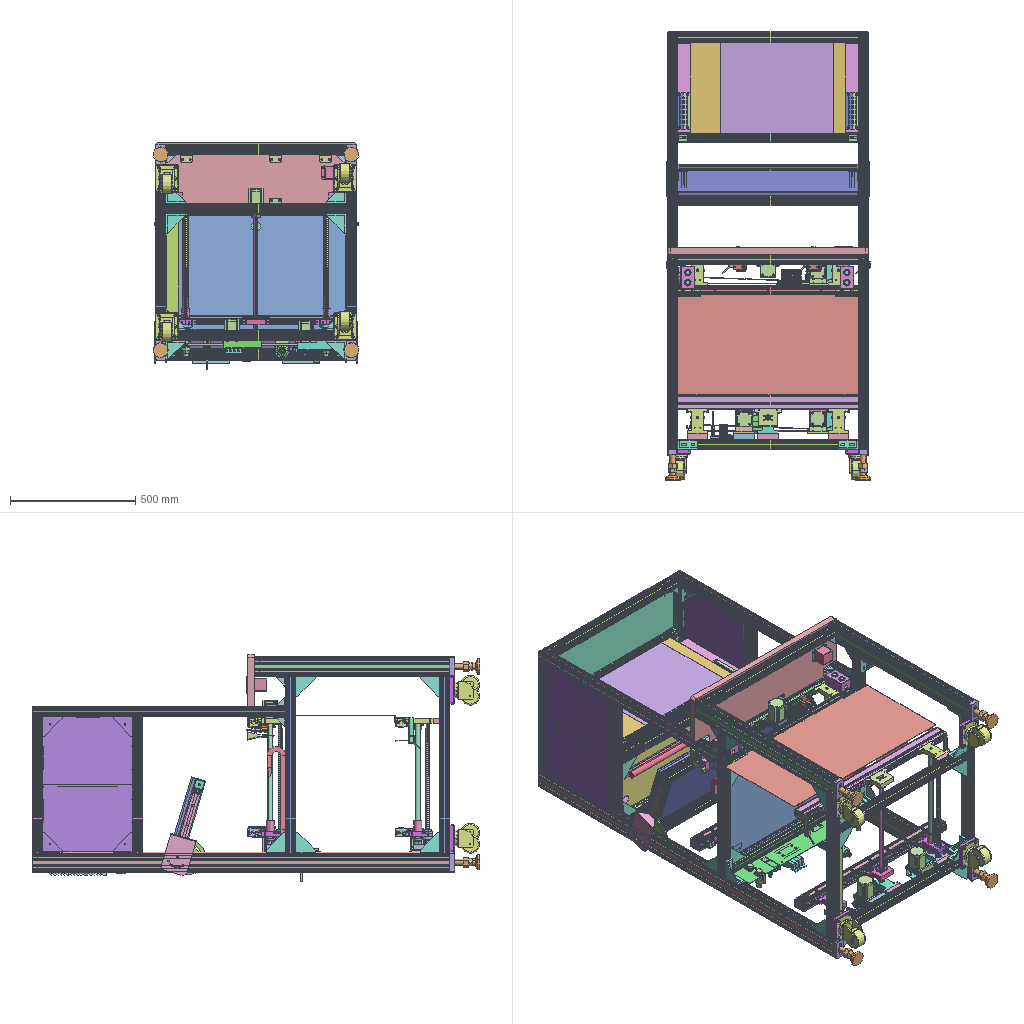Assembly | STEP file | 164 different items | 883 placed | box 820 x 1786 x 902 mm
Parts list (item | name | quantity | parent item | size | volume):
1 | MK-8-4080H-L-02 profile 4080H standard type 1620mm | x2 | in Aluminium profile frame assembly 2 | 1664 x 40 x 80 mm | 1350750 mm3
2 | MK-8-4040C-L-00 profile 4040C standard type 700mm | x4 | in Aluminium profile frame assembly 2 | 700 x 40 x 40 mm | 334774 mm3
3 | MK-8-4040C-L-00 profile 4040C standard type 720mm | x10 | in Aluminium profile frame assembly 2 | 720 x 40 x 40 mm | 344339 mm3
4 | MK-8-4040C-L-00 profile 4040C standard type 540mm | x4 | in Aluminium profile frame assembly 2 | 540 x 40 x 40 mm | 258254 mm3
5 | Die-cast aluminium connector, 40 series, 40mm face, reinforced type | x34 | in Aluminium profile frame assembly 2 | 78 x 78 x 36 mm | 52626 mm3
6 | All-carbon-steel swivel foot KCUF M24-150-60 | x4 | in Aluminium profile frame assembly 2 | 60 x 195 x 60 mm | 136685 mm3
7 | Foot mounting block | x4 | in Aluminium profile frame assembly 2 | 80 x 40 x 20 mm | 52813 mm3
8 | MK-8-4080H-L-02 profile 4080H standard type 735mm | x2 | in Aluminium profile frame assembly 2 | 779 x 40 x 80 mm | 632330 mm3
9 | MK-8-4040C-L-00 profile 4040C standard type 1010mm | x2 | in Aluminium profile frame assembly 2 | 1010 x 40 x 40 mm | 483031 mm3
10 | Die-cast aluminium connector, 40 series, 40mm face, standard type | x18 | in Aluminium profile frame assembly 2 | 38 x 38 x 36 mm | 14409 mm3
11 | 3 inch heavy-duty caster 7223-222B | x4 | in Aluminium profile frame assembly 2 | 112 x 105 x 88 mm | 158459 mm3
12 | Caster mounting plate | x4 | in Aluminium profile frame assembly 2 | 110 x 90 x 14 mm | 130540 mm3
13 | Left door panel | x1 | in Left sheet-metal door assembly | 362.8 x 357 x 19 mm | 160795 mm3
14 | Hinge CL237Z3H001-01 | x4 | in Hinge CL237Z3H001 | 17.5 x 48 x 18 mm | 5234 mm3
15 | Hinge CL237Z3H001-02 | x4 | in Hinge CL237Z3H001 | 19 x 25 x 8.5 mm | 1495 mm3
16 | Power knob mounting sheet metal | x1 | in Left sheet-metal door assembly | 74 x 122 x 41 mm | 24069 mm3
17 | Right door panel | x1 | in Right door welded assembly | 356 x 357 x 17 mm | 169245 mm3
18 | Door hinge mounting plate | x4 | in Frame assembly | 50 x 53 x 16 mm | 6575 mm3
19 | Tabletop mounting plate A | x3 | in Frame assembly | 30 x 36 x 45 mm | 7668 mm3
20 | Cabinet sheet-metal cover plate A | x2 | in Frame assembly | 358 x 30 x 538 mm | 310725 mm3
21 | Power strip mounting plate | x1 | in Frame assembly | 100 x 719 x 60 mm | 188882 mm3
22 | Tabletop plate | x1 | in Frame assembly | 800 x 250 x 27 mm | 5242609 mm3
23 | Lower support plate 1 | x1 | in Frame assembly | 720 x 462 x 30 mm | 565820 mm3
24 | Lower support plate 2 | x1 | in Frame assembly | 52 x 462 x 30 mm | 48079 mm3
25 | Cabinet sheet-metal cover plate B | x1 | in Frame assembly | 794.836 x 358 x 15 mm | 451787 mm3
26 | Top cover plate | x1 | in Frame assembly | 790 x 1.5 x 650 mm | 765787 mm3
27 | Cylinder lock MS813-Shengjiu | x1 | in Frame assembly | 58.793 x 35 x 31.6 mm | 16415 mm3
28 | Class B ventilation filter set ZL-803 (7032 glue) | x2 | in Frame assembly | 150 x 150 x 28 mm | 421271 mm3
29 | Cabinet lower base plate | x1 | in Frame assembly | 718 x 30 x 268 mm | 336091 mm3
30 | Sheet-metal door stop plate | x1 | in Frame assembly | 15.5 x 36.5 x 150 mm | 10828 mm3
31 | Tabletop mounting plate B | x1 | in Frame assembly | 55 x 31 x 45 mm | 10250 mm3
32 | Line stopper plate | x1 | in Frame assembly | 800 x 431 x 30 mm | 516055 mm3
33 | Cabinet brush KEL-BES-S24 | x2 | in Frame assembly | 148 x 10 x 58 mm | 60298 mm3
34 | Electrical mounting plate | x1 | in Control cabinet | 790 x 360 x 20 mm | 612037 mm3
35 | Straight-through terminal block PT2,5-QUATTRO-3209578 | x28 | in Control cabinet | 5.15 x 72.2 x 35.25 mm | 9561 mm3
36 | End clamp-E UK-1201442 | x1 | in Control cabinet | 50.5 x 35.3 x 9.5 mm | 9735 mm3
37 | Miniature circuit breaker IC65N-2P-C16A | x1 | in Control cabinet | 35.4 x 93.9 x 74.3 mm | 159125 mm3
38 | Residual current device Vigi-iC65-ELE-2P-40A-30mA-A | x1 | in Control cabinet | 76.2 x 105.618 x 73.908 mm | 172404 mm3
39 | Power line filter 3ACA5-W33 | x1 | in Control cabinet | 53.2 x 24 x 50 mm | 35444 mm3
40 | Ultra-miniature medium-power relay HF41F_24-ZST and socket 41F-1Z-C2-1 | x1 | in Control cabinet | 88 x 75.5 x 6.1 mm | 25363 mm3
41 | PLC module FX5U-32MT_ES | x1 | in Control cabinet | 150 x 96.4 x 84.9 mm | 980252 mm3
42 | Stepper motor driver DM542-KK V3.0 | x6 | in Control cabinet | 119 x 77.6 x 25.5 mm | 99944 mm3
43 | Cable trough 4 | x2 | in Control cabinet | 50.625 x 25 x 690 mm | 86789 mm3
44 | Cable trough 5 | x2 | in Control cabinet | 50.625 x 25 x 346 mm | 43498 mm3
45 | Power switch LW42B2-1824_L | x1 | in Control cabinet | 65.5 x 92 x 65.5 mm | 250369 mm3
46 | Indicator light AD17-22-AC220VW white | x1 | in Control cabinet | 24 x 37.7 x 24 mm | 7790 mm3
47 | Power supply mounting plate | x2 | in Control cabinet | 65 x 200 x 20 mm | 18055 mm3
48 | Switching power supply LRS-350-24 | x1 | in Control cabinet | 215 x 30 x 115 mm | 695683 mm3
49 | Switching power supply LRS-350-48 | x1 | in Control cabinet | 215 x 30 x 115 mm | 698035 mm3
50 | Primary busbar bracket JTN1 | x2 | in Control cabinet | 20 x 50 x 65 mm | 42874 mm3
51 | Ground copper plate | x1 | in Control cabinet | 30 x 200 x 5 mm | 28923 mm3
52 | Axial fan 1238A2MBL | x1 | in Control cabinet | 120 x 120 x 38 mm | 111801 mm3
53 | Schneider miniature circuit breaker iDPNN-1P+N-C10A | x1 | in Control cabinet | 17.5 x 90.6 x 73.848 mm | 76092 mm3
54 | Schneider AC contactor (coil 24V) LC1D09BDC | x1 | in Control cabinet | - | -
55 | 5-port DIN-rail switch EDS-205 | x1 | in Control cabinet | 98.5 x 110.5 x 24.9 mm | 215104 mm3
56 | Fuse terminal block PT4-HESILED24(5x20)-3211903 | x2 | in Control cabinet | 6.15 x 55.9 x 63.38 mm | 12999 mm3
57 | BZJ-LSX-RGX PLC扩展IO FX5-16ET_ES8(输入,8输出,晶体管漏型) | x1 | in Control cabinet | 40 x 90 x 83 mm | 291482 mm3
58 | Circuit board assembly | x2 | in Control cabinet | 54 x 38 x 11.5 mm | 8666 mm3
59 | T8 integrated LED tube_white 0.6m | x1 | - | 34 x 35.5 x 620 mm | 542828 mm3
60 | Small support plate_sand-blasted, oxidised | x4 | in Forward-flow width-adjust assembly_chain | 20 x 80 x 80 mm | 64176 mm3
61 | Large support plate_sand-blasted, oxidised | x4 | in Forward-flow width-adjust assembly_chain | 20 x 97 x 80 mm | 92738 mm3
62 | Movable support plate_sand-blasted, oxidised | x4 | in Forward-flow width-adjust assembly_chain | 20 x 95 x 90 mm | 73168 mm3
63 | Guide rod | x4 | in Forward-flow width-adjust assembly_chain | 20 x 20 x 505 mm | 158440 mm3
64 | 6001Z bearing stop plate | x4 | in Forward-flow width-adjust assembly_chain | 40 x 28 x 2 mm | 1349 mm3
65 | Bearing stop plate | x5 | in Forward-flow width-adjust assembly_chain, Line single-drive assembly | 40 x 30 x 2 mm | 1364 mm3
66 | Bearing 6000Z_P5_BONA_eco | x5 | in Forward-flow width-adjust assembly_chain, Line single-drive assembly | 26 x 26 x 8 mm | 2544 mm3
67 | Guided double-liner flanged linear bearing LML21-d20 | x4 | in Forward-flow width-adjust assembly_chain | 80 x 54 x 38 mm | 45928 mm3
68 | Nut SFU01604-4 | x4 | in 69 | 40 x 40 x 48 mm | 25660 mm3
69 | Ball screw assembly SFUR1604-545 | x4 | in 69 | 16 x 16 x 545 mm | 99221 mm3
70 | Bearing 6001ZZ | x5 | in Forward-flow width-adjust assembly_chain, Line single-drive assembly | 28 x 28 x 8 mm | 3776 mm3
71 | Locking bearing nut BKN21-M12 (M12×1.0)_yhda | x4 | in Forward-flow width-adjust assembly_chain | 22 x 22 x 8 mm | 1773 mm3
72 | Timing pulley 24-3M-φ10-23 | x4 | in Forward-flow width-adjust assembly_chain | 25 x 23 x 25 mm | 7405 mm3
73 | Motor adapter plate 2 | x2 | in Chain conveyor | 110 x 21 x 64 mm | 49771 mm3
74 | - | x8 | in BZJ-LSX-RGX 链条惰轮Component-30 | 31 x 9 x 31 mm | 3611 mm3
75 | Deep groove ball bearing 606-2Z | x16 | in BZJ-LSX-RGX 链条惰轮Component-30, BZJ-LSX-RGX 链条惰轮Component-25 | 6 x 17 x 17 mm | 776.566 mm3
76 | Internal retaining ring type A 17 | x16 | in BZJ-LSX-RGX 链条惰轮Component-30, BZJ-LSX-RGX 链条惰轮Component-25 | 18.3 x 17.603 x 1 mm | 85.781 mm3
77 | Sprocket spacer | x8 | in Chain conveyor, Line single-drive assembly | 15 x 15 x 6.2 mm | 541.108 mm3
78 | Line rear chain guide rail L800 | x2 | in Chain conveyor, Chain conveyor 2 | 35 x 55 x 800 mm | 614958 mm3
79 | Line front chain guide rail L800 | x1 | in Chain conveyor | 35 x 55 x 800 mm | 614958 mm3
80 | - | x8 | in BZJ-LSX-RGX 链条惰轮Component-25 | 25 x 8.5 x 25 mm | 1521 mm3
81 | Guide rail right end cap | x4 | in Chain conveyor, Chain conveyor 2 | 34.8 x 1 x 54.8 mm | 1804 mm3
82 | Guide rail left end cap | x4 | in Chain conveyor, Chain conveyor 2 | 34.8 x 1 x 54.8 mm | 1804 mm3
83 | 25 small sprocket spacer | x8 | in Chain conveyor, Chain conveyor 2 | 15 x 15 x 3.5 mm | 281.21 mm3
84 | Driven guide wheel connector | x8 | in Chain conveyor, Chain conveyor 2 | 36 x 5 x 10.6 mm | 1667 mm3
85 | Type A plain parallel key GB/T 1096 - key 3x3x12 | x2 | in Chain conveyor | 12 x 3 x 3 mm | 101.479 mm3
86 | BZJ-LSX-RGX 主动链轮06B-10齿_内Holeφ10 | x2 | in Chain conveyor | 34 x 32.715 x 12 mm | 4151 mm3
87 | Stepper motor 24HS8404-10PJ3 | x5 | in Chain conveyor, Belt width-adjust chain conveyor, Belt width-adjust chain conveyor 2, Line single-drive assembly | 60 x 96 x 60 mm | 237550 mm3
88 | Photoelectric sensor mounting plate 2 | x2 | in Chain conveyor | 33 x 38 x 75 mm | 6071 mm3
89 | Retro-reflective photoelectric switch CX-462A | x4 | in Chain conveyor | 30 x 58.715 x 105.315 mm | 11448 mm3
90 | 06B side guide chain support block | x4 | in Chain conveyor, Chain conveyor 2 | 9 x 700 x 20.4 mm | 110428 mm3
91 | 06B side guide chain | x2 | in Chain conveyor, Chain conveyor 2 | 18.325 x 9 x 17.4 mm | 854.513 mm3
92 | 06B side guide chain buckle | x2 | in Chain conveyor, Chain conveyor 2 | 15 x 1 x 7 mm | 49.292 mm3
93 | Polyurethane washer | x4 | in Belt width-adjust chain conveyor, Belt width-adjust chain conveyor 2 | 30 x 13 x 30 mm | 5307 mm3
94 | Photoelectric sensor flag | x2 | in Belt width-adjust chain conveyor, Belt width-adjust chain conveyor 2 | 8 x 40.1 x 11.1 mm | 333.086 mm3
95 | Flanged ball bearing FL626ZZ | x8 | in Driven wheel assembly | 6 x 22 x 22 mm | 1471 mm3
96 | 6mm stainless steel flat washer | x4 | in Driven wheel assembly | 12 x 12 x 1.5 mm | 119.871 mm3
97 | Washer | x4 | in Driven wheel assembly | 15 x 15 x 1.5 mm | 215.297 mm3
98 | Standoff screw φ6x12(M5) | x4 | in Driven wheel assembly | 26.469 x 10 x 10 mm | 868.238 mm3
99 | Washer 2 | x4 | in Driven wheel assembly | 9.5 x 9.5 x 1.6 mm | 63.536 mm3
100 | Washer A | x4 | in Driven wheel assembly | 12 x 1 x 12 mm | 79.914 mm3
101 | Timing pulley 16-3M-Φ10-18 | x3 | in Belt width-adjust chain conveyor, Belt width-adjust chain conveyor 2, Line single-drive assembly | 17.5 x 18 x 17.5 mm | 1873 mm3
102 | Motor adapter plate A | x2 | in Belt width-adjust chain conveyor, Belt width-adjust chain conveyor 2 | 84 x 40 x 86 mm | 49205 mm3
103 | Motor support plate | x3 | in Belt width-adjust chain conveyor, Belt width-adjust chain conveyor 2, Line single-drive assembly | 11.5 x 65 x 65 mm | 12844 mm3
104 | Belt guard | x2 | in Belt width-adjust chain conveyor, Belt width-adjust chain conveyor 2 | 135 x 87.5 x 48 mm | 32458 mm3
105 | Timing belt 1293-3M-9mm wide | x2 | in Belt width-adjust chain conveyor, Belt width-adjust chain conveyor 2 | 588.86 x 60.04 x 9 mm | 23269 mm3
106 | 06B side guide chain | x354 | in Belt width-adjust chain conveyor | 18.325 x 9 x 17.4 mm | 854.513 mm3
107 | Pressure regulating filter GFR300-08-N | x1 | - | - | -
108 | I/O distribution box 23N8S1 | x1 | - | - | -
109 | Plug (straight male) | x12 | - | - | -
110 | Line front chain guide rail 800 | x1 | in Chain conveyor 2 | 35 x 55 x 800 mm | 614958 mm3
111 | CX440 adjusting plate 2_powder-coated matt silver grey | x2 | in Chain conveyor 2 | 18.5 x 102 x 16 mm | 4317 mm3
112 | Compact photoelectric sensor CX-441 | x2 | in Chain conveyor 2 | 11.2 x 58.715 x 100.215 mm | 7246 mm3
113 | Bearing mounting plate A | x1 | in Line single-drive assembly | 110 x 68 x 20 mm | 88933 mm3
114 | 36-3M-φ10-19-J timing pulley | x1 | in Line single-drive assembly | 37 x 19 x 37 mm | 15386 mm3
115 | - | x1 | in Line single-drive assembly | 122.93 x 36.98 x 8 mm | 5373 mm3
116 | BZJ-LSX-RGX 主动链轮06B-15齿_内Holeφ16 | x1 | in Line single-drive assembly | 50.395 x 50.132 x 19 mm | 15455 mm3
117 | Bearing 6904Z | x1 | in Line single-drive assembly | 9 x 37 x 37 mm | 4601 mm3
118 | Drive shaft sleeve | x1 | in Line single-drive assembly | 23 x 23 x 31.4 mm | 3535 mm3
119 | BZJ-LSX-RGX 主动链轮06B-15齿_内Holeφ20_J | x1 | in Line single-drive assembly | 50.395 x 50.132 x 19.5 mm | 13040 mm3
120 | Bearing mounting plate 2 | x1 | in Line single-drive assembly | 110 x 68 x 20 mm | 100152 mm3
121 | Drive shaft 2 | x1 | in Line single-drive assembly | 16 x 544 x 16 mm | 100395 mm3
122 | Small support plate A | x1 | in Line single-drive assembly | 20 x 80 x 80 mm | 68710 mm3
123 | Motor adapter plate | x1 | in Line single-drive assembly | 84 x 32 x 86 mm | 43828 mm3
124 | Key 2 | x1 | in Line single-drive assembly | 3.9 x 5.5 x 15 mm | 300.753 mm3
125 | Belt guard A | x1 | in Belt width-adjust chain conveyor 2 | 150 x 86 x 40 mm | 33822 mm3
126 | Riser plate_sand-blasted, oxidised | x5 | in Belt width-adjust chain conveyor 2 | 20 x 26 x 80 mm | 39834 mm3
127 | Riser plate 4_sand-blasted, oxidised | x1 | in Belt width-adjust chain conveyor 2 | 20 x 26 x 87 mm | 43474 mm3
128 | Stopper bar limit plate | x2 | in Stopper assembly_front | 12.5 x 39 x 70 mm | 17639 mm3
129 | Stopper bar | x2 | in Stopper assembly_front | 14 x 5 x 94 mm | 6342 mm3
130 | Stopper bar cover plate | x2 | in Stopper assembly_front | 70 x 4 x 38 mm | 9112 mm3
131 | Cylinder mounting plate | x2 | in Stopper assembly_front | 38 x 32 x 38 mm | 17881 mm3
132 | M3x8 socket head cap screw | x14 | in Stopper assembly_front | 5.5 x 11 x 5.5 mm | 105.547 mm3
133 | Miniature tube fitting M-3ALU-4 | x4 | in Stopper assembly_front | 5 x 9.5 x 10.687 mm | 200.167 mm3
134 | Compact free-mount cylinder MU10x10S | x2 | in Stopper assembly_front | 34 x 22 x 13.5 mm | 6493 mm3
135 | Height-limit steel tube | x2 | in Stopper assembly_front | 4 x 4 x 4.1 mm | 14.297 mm3
136 | Stopper bar mounting plate | x2 | in Stopper assembly_front | 19 x 37 x 4 mm | 1217 mm3
137 | Cable carrier support plate C | x1 | - | 30 x 50 x 30 mm | 4308 mm3
138 | Cable carrier J15BF.1.20N28 | x1 | - | 28.5 x 74.5 x 367.25 mm | 251972 mm3
139 | Photoelectric sensor PM-Y65 | x2 | - | 22.7 x 14.9 x 13.4 mm | 1660 mm3
140 | Push button box mounting base plate | x2 | in Width-adjust push button box assembly | 52 x 2 x 102 mm | 10204 mm3
141 | Push button housing | x2 | in Width-adjust push button box assembly | 55 x 45 x 90 mm | 16840 mm3
142 | Metal push button switch ring light GQ22-L-11E_G_24V_S | x3 | in Width-adjust push button box assembly | 28.5 x 25 x 38.7 mm | 12469 mm3
143 | Metal push button switch ring light GQ22-L-11E_Y_24V_S | x2 | in Width-adjust push button box assembly | 28.5 x 25 x 38.7 mm | 12469 mm3
144 | Solenoid valve base 7V100M4F | x1 | - | 23 x 57.5 x 88 mm | 80180 mm3
145 | Solenoid valve 7V130C06B-NS | x4 | - | 141.7 x 32.5 x 16 mm | 47379 mm3
146 | I/O distribution box 23N4S1 | x2 | - | 29.939 x 86.939 x 25.75 mm | 38975 mm3
147 | 982 plug (1-8 plug) | x3 | - | 10 x 6.95 x 10 mm | 421.396 mm3
148 | BZJ-LSX-RGX M8分配器电缆6端口8芯Vertical出线3米(PVC)64S423-030 | x3 | - | 99 x 14.979 x 14.996 mm | 5984 mm3
149 | Manual slide valve HSV08 | x1 | - | - | -
150 | External hex shaft joint APH8-02 | x1 | - | 37.183 x 28 x 17.166 mm | 6274 mm3
151 | SMEMA connector | x4 | - | 36 x 36 x 78.52 mm | 45655 mm3
152 | Push button switch guard | x1 | - | 78 x 50 x 50 mm | 13195 mm3
153 | Push button switch mounting plate 2 | x1 | - | 70 x 70 x 3 mm | 12912 mm3
154 | MK-8-4040C-L-00 profile 4040C standard type 1270mm | x2 | in Magazine bracket assembly | 720 x 40 x 40 mm | 346595 mm3
155 | MK-8-4040C-L-00 profile 4040C standard type 400mm | x2 | in Magazine bracket assembly | 300 x 40 x 40 mm | 143475 mm3
156 | End cap panel MK-EC-B-4040x4.2 | x4 | in Magazine bracket assembly | 40 x 12.4 x 40 mm | 5038 mm3
157 | New in-slot right-angle connector, 40 series (with set screw) | x4 | in Magazine bracket assembly | 38 x 31 x 18.5 mm | 6406 mm3
158 | Magazine plate | x1 | - | 717 x 380 x 20 mm | 394457 mm3
159 | Magazine bracket mounting plate | x2 | - | 140 x 90 x 40 mm | 42824 mm3
160 | Tray bracket support plate | x2 | - | 328 x 106 x 43 mm | 74121 mm3
161 | 01.1.015030-L-00 magazine hanger profile 15x30-1269 | x2 | - | 720 x 30 x 15 mm | 154915 mm3
162 | Kanban base plate | x1 | - | 620 x 386 x 2 mm | 478633 mm3
163 | PC board | x1 | - | 386 x 450 x 1 mm | 173679 mm3
164 | Kanban profile mounting bracket | x4 | - | 40 x 65 x 30 mm | 8738 mm3
Placements (level | parent | child | x y z in mm | rotation matrix by rows), first 283 of 928 lines:
1 | subassembly 2 | Frame assembly | -0.0 0.0 -0.0 | 1 0 0 0 1 0 0 0 1
2 | Frame assembly | Aluminium profile frame assembly 2 | 877.856 282.252 1817.393 | 1 0 0 0 1 0 0 0 1
3 | Aluminium profile frame assembly 2 | MK-8-4080H-L-02 profile 4080H standard type 1620mm | 0.0 -0.0 -0.0 | 0 -1 0 -1 0 0 0 0 -1
3 | Aluminium profile frame assembly 2 | MK-8-4080H-L-02 profile 4080H standard type 1620mm | 760.0 0.0 0.0 | 0 -1 0 -1 0 0 0 0 -1
3 | Aluminium profile frame assembly 2 | MK-8-4040C-L-00 profile 4040C standard type 700mm | 760.0 -1644.0 40 | 0 -1 0 0 0 -1 1 0 -0
3 | Aluminium profile frame assembly 2 | MK-8-4040C-L-00 profile 4040C standard type 720mm | 20.0 -905.0 800 | 1 0 0 0 0 -1 0 1 -0
3 | Aluminium profile frame assembly 2 | MK-8-4040C-L-00 profile 4040C standard type 700mm | 0.0 -1644.0 40 | 0 -1 0 0 0 -1 1 0 -0
3 | Aluminium profile frame assembly 2 | MK-8-4040C-L-00 profile 4040C standard type 720mm | 20.0 -1644.0 564 | 1 0 0 0 0 -1 0 1 -0
3 | Aluminium profile frame assembly 2 | MK-8-4040C-L-00 profile 4040C standard type 720mm | 20.0 -1644.0 60 | 1 0 0 0 0 -1 0 1 -0
3 | Aluminium profile frame assembly 2 | MK-8-4040C-L-00 profile 4040C standard type 540mm | 0.0 -20.0 40 | 0 0 1 0 -1 0 1 0 -0
3 | Aluminium profile frame assembly 2 | MK-8-4040C-L-00 profile 4040C standard type 540mm | 760.0 -20.0 40 | 0 0 1 0 -1 0 1 0 -0
3 | Aluminium profile frame assembly 2 | MK-8-4040C-L-00 profile 4040C standard type 720mm | 740.0 -20.0 -20 | -1 0 0 0 1 0 0 0 -1
3 | Aluminium profile frame assembly 2 | MK-8-4040C-L-00 profile 4040C standard type 720mm | 740.0 -420.0 -20 | -1 0 0 0 1 0 0 0 -1
3 | Aluminium profile frame assembly 2 | MK-8-4040C-L-00 profile 4040C standard type 540mm | 0.0 -420.0 40 | 0 0 1 0 -1 0 1 0 -0
3 | Aluminium profile frame assembly 2 | MK-8-4040C-L-00 profile 4040C standard type 540mm | 760.0 -420.0 40 | 0 0 1 0 -1 0 1 0 -0
3 | Aluminium profile frame assembly 2 | MK-8-4040C-L-00 profile 4040C standard type 700mm | 0.0 -1030.0 40 | 0 -1 0 0 0 -1 1 0 -0
3 | Aluminium profile frame assembly 2 | MK-8-4040C-L-00 profile 4040C standard type 700mm | 760.0 -1030.0 40 | 0 -1 0 0 0 -1 1 0 -0
3 | Aluminium profile frame assembly 2 | MK-8-4040C-L-00 profile 4040C standard type 720mm | 740.0 -1030.0 60 | -1 0 0 0 0 1 0 1 0
3 | Aluminium profile frame assembly 2 | MK-8-4040C-L-00 profile 4040C standard type 720mm | 740.0 -1030.0 564 | -1 0 0 0 0 1 0 1 0
3 | Aluminium profile frame assembly 2 | MK-8-4040C-L-00 profile 4040C standard type 720mm | 20.0 -20.0 600 | 1 0 0 0 0 -1 0 1 0
3 | Aluminium profile frame assembly 2 | Die-cast aluminium connector, 40 series, 40mm face, reinforced type | 20.0 -1662.0 584 | 0 1 0 0 0 1 1 0 0
3 | Aluminium profile frame assembly 2 | Die-cast aluminium connector, 40 series, 40mm face, reinforced type | 740.0 -1662.0 584 | -1 0 0 0 0 1 0 1 0
3 | Aluminium profile frame assembly 2 | Die-cast aluminium connector, 40 series, 40mm face, reinforced type | 740.0 -1662.0 40 | 0 -1 0 0 0 1 -1 0 0
3 | Aluminium profile frame assembly 2 | Die-cast aluminium connector, 40 series, 40mm face, reinforced type | 20.0 -1662.0 40 | 1 0 0 0 0 1 0 -1 0
3 | Aluminium profile frame assembly 2 | Die-cast aluminium connector, 40 series, 40mm face, reinforced type | -18.0 -1050.0 740 | 0 0 1 -1 0 0 0 -1 0
3 | Aluminium profile frame assembly 2 | Die-cast aluminium connector, 40 series, 40mm face, reinforced type | -18.0 -1050.0 40 | 0 0 1 0 -1 0 1 0 0
3 | Aluminium profile frame assembly 2 | Die-cast aluminium connector, 40 series, 40mm face, reinforced type | 20.0 -1662.0 544 | 1 0 0 0 0 1 0 -1 0
3 | Aluminium profile frame assembly 2 | Die-cast aluminium connector, 40 series, 40mm face, reinforced type | 20.0 -1662.0 80 | 0 1 0 0 0 1 1 0 0
3 | Aluminium profile frame assembly 2 | Die-cast aluminium connector, 40 series, 40mm face, reinforced type | 740.0 -1662.0 544 | 0 -1 0 0 0 1 -1 0 0
3 | Aluminium profile frame assembly 2 | Die-cast aluminium connector, 40 series, 40mm face, reinforced type | 740.0 -1662.0 80 | -1 0 0 0 0 1 0 1 0
3 | Aluminium profile frame assembly 2 | Die-cast aluminium connector, 40 series, 40mm face, reinforced type | 778.0 -1010.0 40 | 0 0 -1 0 1 0 1 0 0
3 | Aluminium profile frame assembly 2 | Die-cast aluminium connector, 40 series, 40mm face, reinforced type | 778.0 -1624.0 40 | 0 0 -1 0 1 0 1 0 0
3 | Aluminium profile frame assembly 2 | Die-cast aluminium connector, 40 series, 40mm face, reinforced type | 778.0 -1050.0 40 | 0 0 -1 -1 0 0 0 1 0
3 | Aluminium profile frame assembly 2 | Die-cast aluminium connector, 40 series, 40mm face, reinforced type | 778.0 -1050.0 740 | 0 0 -1 0 -1 0 -1 0 0
3 | Aluminium profile frame assembly 2 | Die-cast aluminium connector, 40 series, 40mm face, reinforced type | -18.0 -1624.0 40 | 0 0 1 1 0 0 0 1 0
3 | Aluminium profile frame assembly 2 | Die-cast aluminium connector, 40 series, 40mm face, reinforced type | -18.0 -1624.0 740 | 0 0 1 0 1 0 -1 0 0
3 | Aluminium profile frame assembly 2 | Die-cast aluminium connector, 40 series, 40mm face, reinforced type | 778.0 -1624.0 740 | 0 0 -1 1 0 0 0 -1 0
3 | Aluminium profile frame assembly 2 | All-carbon-steel swivel foot KCUF M24-150-60 | 0.0 -1784.0 0.0001 | 0.4085 0 -0.9127 0 1 0 0.9127 0 0.4085
3 | Aluminium profile frame assembly 2 | All-carbon-steel swivel foot KCUF M24-150-60 | 0.0 -1784.0 780 | 0.5097 0 0.8604 0 1 0 -0.8604 0 0.5097
3 | Aluminium profile frame assembly 2 | All-carbon-steel swivel foot KCUF M24-150-60 | 760.0 -1784.0 780 | -0.6285 0 -0.7778 0 1 0 0.7778 0 -0.6285
3 | Aluminium profile frame assembly 2 | All-carbon-steel swivel foot KCUF M24-150-60 | 760.0 -1784.0 0.0001 | 0.4445 0 0.8958 0 1 0 -0.8958 0 0.4445
3 | Aluminium profile frame assembly 2 | Die-cast aluminium connector, 40 series, 40mm face, reinforced type | -18.0 -1010.0 40 | 0 0 1 1 0 0 0 1 -0
3 | Aluminium profile frame assembly 2 | Foot mounting block | 0.0 -1664.0 0.0001 | 0 -1 0 0 0 -1 1 0 0
3 | Aluminium profile frame assembly 2 | Foot mounting block | 0.0 -1664.0 780 | 0 -1 0 0 0 -1 1 0 -0
3 | Aluminium profile frame assembly 2 | Foot mounting block | 760.0 -1664.0 780 | 0 -1 0 0 0 -1 1 0 -0
3 | Aluminium profile frame assembly 2 | Foot mounting block | 760.0 -1664.0 0.0001 | 0 -1 0 0 0 -1 1 0 -0
3 | Aluminium profile frame assembly 2 | MK-8-4080H-L-02 profile 4080H standard type 735mm | -0.0 -885.0 780 | 0 -1 0 -1 0 0 0 0 -1
3 | Aluminium profile frame assembly 2 | MK-8-4080H-L-02 profile 4080H standard type 735mm | 760.0 -885.0 780 | 0 -1 0 -1 0 0 0 0 -1
3 | Aluminium profile frame assembly 2 | MK-8-4040C-L-00 profile 4040C standard type 1010mm | 0.0 -1010.0 600 | 0 -1 0 1 0 0 0 0 1
3 | Aluminium profile frame assembly 2 | MK-8-4040C-L-00 profile 4040C standard type 1010mm | 760.0 -1010.0 600 | 0 -1 0 1 0 0 0 0 1
3 | Aluminium profile frame assembly 2 | MK-8-4040C-L-00 profile 4040C standard type 720mm | 740.0 -420.0 290 | -1 0 0 0 1 0 0 0 -1
3 | Aluminium profile frame assembly 2 | MK-8-4040C-L-00 profile 4040C standard type 720mm | 20.0 -20.0 290 | 1 0 0 0 0 -1 0 1 0
3 | Aluminium profile frame assembly 2 | Die-cast aluminium connector, 40 series, 40mm face, reinforced type | -18.0 -40.0 40 | 0 0 1 0 -1 0 1 0 -0
3 | Aluminium profile frame assembly 2 | Die-cast aluminium connector, 40 series, 40mm face, reinforced type | -18.0 -400.0 40 | 0 0 1 1 0 0 0 1 -0
3 | Aluminium profile frame assembly 2 | Die-cast aluminium connector, 40 series, 40mm face, reinforced type | -18.0 -40.0 580 | 0 0 1 -1 0 0 0 -1 -0
3 | Aluminium profile frame assembly 2 | Die-cast aluminium connector, 40 series, 40mm face, reinforced type | -18.0 -400.0 580 | 0 0 1 0 1 0 -1 0 0
3 | Aluminium profile frame assembly 2 | Die-cast aluminium connector, 40 series, 40mm face, reinforced type | 778.0 -40.0 580 | 0 0 -1 0 -1 0 -1 0 -0
3 | Aluminium profile frame assembly 2 | Die-cast aluminium connector, 40 series, 40mm face, reinforced type | 778.0 -400.0 580 | 0 0 -1 1 0 0 0 -1 -0
3 | Aluminium profile frame assembly 2 | Die-cast aluminium connector, 40 series, 40mm face, reinforced type | 778.0 -40.0 40 | 0 0 -1 -1 0 0 0 1 -0
3 | Aluminium profile frame assembly 2 | Die-cast aluminium connector, 40 series, 40mm face, reinforced type | 778.0 -400.0 40 | 0 0 -1 0 1 0 1 0 -0
3 | Aluminium profile frame assembly 2 | Die-cast aluminium connector, 40 series, 40mm face, reinforced type | 20.0 -438.0 270 | 1 0 0 0 0 1 0 -1 -0
3 | Aluminium profile frame assembly 2 | Die-cast aluminium connector, 40 series, 40mm face, reinforced type | 740.0 -438.0 0.0001 | -1 0 0 0 0 1 0 1 -0
3 | Aluminium profile frame assembly 2 | Die-cast aluminium connector, 40 series, 40mm face, reinforced type | 20.0 -438.0 0.0001 | 0 1 0 0 0 1 1 0 -0
3 | Aluminium profile frame assembly 2 | Die-cast aluminium connector, 40 series, 40mm face, reinforced type | 740.0 -438.0 270 | 0 -1 0 0 0 1 -1 0 -0
3 | Aluminium profile frame assembly 2 | Die-cast aluminium connector, 40 series, 40mm face, standard type | 20.0 -20.0 580 | 1 0 0 0 0 1 0 -1 -0
3 | Aluminium profile frame assembly 2 | Die-cast aluminium connector, 40 series, 40mm face, standard type | 740.0 -20.0 580 | 0 -1 0 0 0 1 -1 0 0
3 | Aluminium profile frame assembly 2 | Die-cast aluminium connector, 40 series, 40mm face, standard type | 740.0 -20.0 310 | -1 0 0 0 0 1 0 1 -0
3 | Aluminium profile frame assembly 2 | Die-cast aluminium connector, 40 series, 40mm face, standard type | 20.0 -20.0 310 | 0 1 0 0 0 1 1 0 -0
3 | Aluminium profile frame assembly 2 | Die-cast aluminium connector, 40 series, 40mm face, standard type | 740.0 -20.0 270 | 0 -1 0 0 0 1 -1 0 0
3 | Aluminium profile frame assembly 2 | Die-cast aluminium connector, 40 series, 40mm face, standard type | 20.0 -20.0 270 | 1 0 0 0 0 1 0 -1 -0
3 | Aluminium profile frame assembly 2 | Die-cast aluminium connector, 40 series, 40mm face, standard type | 20.0 -20.0 0.0001 | 1 0 0 0 0 -1 0 1 0
3 | Aluminium profile frame assembly 2 | Die-cast aluminium connector, 40 series, 40mm face, standard type | 740.0 -20.0 0.0001 | 0 -1 0 0 0 -1 1 0 -0
3 | Aluminium profile frame assembly 2 | Die-cast aluminium connector, 40 series, 40mm face, reinforced type | 740.0 -1048.0 80 | -1 0 0 0 0 1 0 1 0
3 | Aluminium profile frame assembly 2 | Die-cast aluminium connector, 40 series, 40mm face, reinforced type | 740.0 -1048.0 544 | 0 -1 0 0 0 1 -1 0 0
3 | Aluminium profile frame assembly 2 | Die-cast aluminium connector, 40 series, 40mm face, reinforced type | 20.0 -1048.0 80 | 0 1 0 0 0 1 1 0 0
3 | Aluminium profile frame assembly 2 | Die-cast aluminium connector, 40 series, 40mm face, reinforced type | 20.0 -1048.0 544 | 1 0 0 0 0 1 0 -1 0
3 | Aluminium profile frame assembly 2 | Die-cast aluminium connector, 40 series, 40mm face, standard type | 760.0 -1010.0 580 | 0 0 1 0 1 0 -1 0 -0
3 | Aluminium profile frame assembly 2 | Die-cast aluminium connector, 40 series, 40mm face, standard type | 760.0 -1010.0 620 | 0 0 -1 0 1 0 1 0 0
3 | Aluminium profile frame assembly 2 | Die-cast aluminium connector, 40 series, 40mm face, standard type | 0.0 -1010.0 580 | 0 0 1 0 1 0 -1 0 -0
3 | Aluminium profile frame assembly 2 | Die-cast aluminium connector, 40 series, 40mm face, standard type | 0.0 -1010.0 620 | 0 0 -1 0 1 0 1 0 0
3 | Aluminium profile frame assembly 2 | Die-cast aluminium connector, 40 series, 40mm face, standard type | 760.0 -1010.0 740 | 0 0 1 0 1 0 -1 0 -0
3 | Aluminium profile frame assembly 2 | Die-cast aluminium connector, 40 series, 40mm face, standard type | 0.0 -1010.0 740 | 0 0 1 0 1 0 -1 0 -0
3 | Aluminium profile frame assembly 2 | Die-cast aluminium connector, 40 series, 40mm face, standard type | 740.0 -885.0 600 | 0 -1 0 -1 0 0 0 0 -1
3 | Aluminium profile frame assembly 2 | Die-cast aluminium connector, 40 series, 40mm face, standard type | 20.0 -885.0 600 | 0 1 0 -1 0 0 0 0 1
3 | Aluminium profile frame assembly 2 | 3 inch heavy-duty caster 7223-222B | 735.0 -1683.0 95 | 0 0 1 0 1 0 -1 0 0
3 | Aluminium profile frame assembly 2 | Caster mounting plate | 735.0 -1664.0 95 | 0 -1 0 0 0 -1 1 0 -0
3 | Aluminium profile frame assembly 2 | 3 inch heavy-duty caster 7223-222B | 25.0 -1683.0 685 | 0 0 -1 0 1 0 1 0 -0
3 | Aluminium profile frame assembly 2 | Caster mounting plate | 25.0 -1664.0 685 | 0 1 0 0 0 -1 -1 0 -0
3 | Aluminium profile frame assembly 2 | 3 inch heavy-duty caster 7223-222B | 25.0 -1683.0 95 | 0 0 -1 0 1 0 1 0 -0
3 | Aluminium profile frame assembly 2 | Caster mounting plate | 25.0 -1664.0 95 | 0 1 0 0 0 -1 -1 0 -0
3 | Aluminium profile frame assembly 2 | 3 inch heavy-duty caster 7223-222B | 735.0 -1683.0 685 | 0 0 1 0 1 0 -1 0 0
3 | Aluminium profile frame assembly 2 | Caster mounting plate | 735.0 -1664.0 685 | 0 -1 0 0 0 -1 1 0 -0
3 | Aluminium profile frame assembly 2 | Die-cast aluminium connector, 40 series, 40mm face, standard type | 740.0 -905.0 780 | 0 -1 0 0 0 1 -1 0 0
3 | Aluminium profile frame assembly 2 | Die-cast aluminium connector, 40 series, 40mm face, standard type | 20.0 -905.0 780 | 0 1 0 0 0 -1 -1 0 -0
2 | Frame assembly | Left sheet-metal door assembly | 1035.277 105.718 2093.494 | -1 0 0 0 -1 0 0 0 1
3 | Left sheet-metal door assembly | Left door panel | -402.579 43.466 -315.1 | -1 0 0 0 -1 0 0 0 1
3 | Left sheet-metal door assembly | Hinge CL237Z3H001 | -549.398 -101.165 -270.668 | -1 0 0 0 1 0 0 0 -1
4 | Hinge CL237Z3H001 | Hinge CL237Z3H001-01 | 25.631 24.631 40.182 | 1 0 0 0 1 0 0 0 1
4 | Hinge CL237Z3H001 | Hinge CL237Z3H001-02 | 25.631 24.631 40.182 | -1 0 0 0 1 0 0 0 -1
3 | Left sheet-metal door assembly | Hinge CL237Z3H001 | -549.398 138.835 -270.668 | -1 0 0 0 1 0 0 0 -1
4 | Hinge CL237Z3H001 | Hinge CL237Z3H001-01 | 25.631 24.631 40.182 | 1 0 0 0 1 0 0 0 1
4 | Hinge CL237Z3H001 | Hinge CL237Z3H001-02 | 25.631 24.631 40.182 | -1 0 0 0 1 0 0 0 -1
3 | Left sheet-metal door assembly | Power knob mounting sheet metal | -382.579 122.966 -274.1 | -1 0 0 0 -1 0 0 0 1
2 | Frame assembly | Right door welded assembly | 1480.436 18.785 2093.494 | 1 0 0 0 1 0 0 0 1
3 | Right door welded assembly | Right door panel | -402.579 43.466 -315.1 | -1 0 0 0 -1 0 0 0 1
3 | Right door welded assembly | Hinge CL237Z3H001 | -549.398 -101.165 -270.668 | -1 0 0 0 1 0 0 0 -1
4 | Hinge CL237Z3H001 | Hinge CL237Z3H001-01 | 25.631 24.631 40.182 | 1 0 0 0 1 0 0 0 1
4 | Hinge CL237Z3H001 | Hinge CL237Z3H001-02 | 25.631 24.631 40.182 | -1 0 0 0 1 0 0 0 -1
3 | Right door welded assembly | Hinge CL237Z3H001 | -549.398 138.835 -270.668 | -1 0 0 0 1 0 0 0 -1
4 | Hinge CL237Z3H001 | Hinge CL237Z3H001-01 | 25.631 24.631 40.182 | 1 0 0 0 1 0 0 0 1
4 | Hinge CL237Z3H001 | Hinge CL237Z3H001-02 | 25.631 24.631 40.182 | -1 0 0 0 1 0 0 0 -1
2 | Frame assembly | Door hinge mounting plate | 899.356 182.252 1822.893 | 0 0 1 -1 0 0 0 -1 0
2 | Frame assembly | Door hinge mounting plate | 899.356 -57.748 1822.893 | 0 0 1 -1 0 0 0 -1 0
2 | Frame assembly | Door hinge mounting plate | 1616.356 182.252 1822.893 | 0 0 -1 1 0 0 0 -1 0
2 | Frame assembly | Door hinge mounting plate | 1616.356 -57.748 1822.893 | 0 0 -1 1 0 0 0 -1 0
2 | Frame assembly | Tabletop mounting plate A | 1535.356 -602.748 2567.393 | 0 0 -1 0 1 0 1 0 0
2 | Frame assembly | Tabletop mounting plate A | 980.356 -602.748 2567.393 | 0 0 -1 0 1 0 1 0 0
2 | Frame assembly | Cabinet sheet-metal cover plate A | 858.356 62.252 2127.393 | 0 -1 0 -1 0 0 0 0 -1
2 | Frame assembly | Cabinet sheet-metal cover plate A | 1657.356 62.252 2127.393 | 0 1 0 1 0 0 0 0 -1
2 | Frame assembly | Power strip mounting plate | 1617.356 -767.748 1859.393 | 0 -1 0 -1 0 0 0 0 -1
2 | Frame assembly | Tabletop plate | 1257.856 -602.748 2518.893 | 1 0 0 0 0 1 0 -1 0
2 | Frame assembly | Tabletop mounting plate A | 1335.356 -602.748 2567.393 | 0 0 -1 0 1 0 1 0 0
2 | Frame assembly | Lower support plate 1 | 1257.856 -727.748 2129.393 | -1 0 0 0 0 1 0 1 0
2 | Frame assembly | Lower support plate 2 | 1257.856 -1341.748 2129.393 | -1 0 0 0 0 1 0 1 -0
2 | Frame assembly | Cabinet sheet-metal cover plate B | 1257.856 61.252 2127.394 | -1 0 0 0 -1 0 0 0 1
2 | Frame assembly | Top cover plate | 1257.856 283.752 2107.393 | 1 0 0 0 1 0 0 0 1
2 | Frame assembly | Cylinder lock MS813-Shengjiu | 1218.856 -68.248 1777.194 | 1 0 0 0 -1 0 0 0 -1
2 | Frame assembly | Class B ventilation filter set ZL-803 (7032 glue) | 1077.856 62.252 1764.194 | -1 0 0 0 1 0 0 0 -1
2 | Frame assembly | Cabinet lower base plate | 1257.856 -117.748 1952.393 | 1 0 0 0 1 0 0 0 1
2 | Frame assembly | Sheet-metal door stop plate | 1182.856 -116.248 1833.393 | 0 0 1 1 0 0 0 1 -0
2 | Frame assembly | Tabletop mounting plate B | 1335.356 -602.748 2423.893 | 0 0 1 0 1 0 -1 0 -0
2 | Frame assembly | Line stopper plate | 1257.856 -947.498 2402.893 | 1 0 0 0 1 0 0 0 1
2 | Frame assembly | Cabinet brush KEL-BES-S24 | 1594.856 -31.748 2137.394 | 0 0 1 -1 0 0 0 -1 0
2 | Frame assembly | Cabinet brush KEL-BES-S24 | 920.856 -31.748 2137.394 | 0 0 1 -1 0 0 0 -1 0
2 | Frame assembly | Class B ventilation filter set ZL-803 (7032 glue) | 1437.856 140.752 1764.194 | -1 0 0 0 1 0 0 0 -1
1 | subassembly 2 | Control cabinet | 1258.856 -117.748 2097.394 | -1 0 0 0 1 0 0 0 -1
2 | Control cabinet | Electrical mounting plate | -0.0 -0.0 -0.0 | 1 0 0 0 1 0 0 0 1
2 | Control cabinet | Straight-through terminal block PT2,5-QUATTRO-3209578 | 162.15 204.05 2.0 | 1 0 0 0 1 0 0 0 1
2 | Control cabinet | End clamp-E UK-1201442 | 167.3 157.158 -83.581 | 0 0 1 1 0 0 0 1 -0
2 | Control cabinet | Miniature circuit breaker IC65N-2P-C16A | -302.05 197.696 73.435 | 1 0 0 0 1 0 0 0 1
2 | Control cabinet | Residual current device Vigi-iC65-ELE-2P-40A-30mA-A | -284.35 191.696 73.076 | 1 0 0 0 1 0 0 0 1
2 | Control cabinet | Straight-through terminal block PT2,5-QUATTRO-3209578 | -324.2 204.05 2.0 | 1 0 0 0 1 0 0 0 1
2 | Control cabinet | Power line filter 3ACA5-W33 | -264.5 76.1 2.0 | 0 0 -1 -1 0 0 0 1 0
2 | Control cabinet | Ultra-miniature medium-power relay HF41F_24-ZST and socket 41F-1Z-C2-1 | 179.85 239.564 2.0 | 0 0 1 1 0 0 0 1 0
2 | Control cabinet | PLC module FX5U-32MT_ES | -139.8 209.0 2.0 | 1 0 0 0 1 0 0 0 1
2 | Control cabinet | Stepper motor driver DM542-KK V3.0 | -52.3 70.0 77.5 | 0 0 1 -1 0 0 0 -1 -0
2 | Control cabinet | Cable trough 4 | -0.0 152.5 2.0 | 0 0 1 0 -1 0 1 0 0
2 | Control cabinet | Cable trough 4 | -0.0 345.5 2.0 | 0 0 1 0 -1 0 1 0 -0
2 | Control cabinet | Cable trough 5 | -357.5 183.0 2.0 | 0 -1 0 0 0 -1 1 0 0
2 | Control cabinet | Cable trough 5 | 362.5 183.0 2.0 | 0 -1 0 0 0 -1 1 0 -0
2 | Control cabinet | Straight-through terminal block PT2,5-QUATTRO-3209578 | 156.35 204.05 2.0 | 1 0 0 0 1 0 0 0 1
2 | Control cabinet | Straight-through terminal block PT2,5-QUATTRO-3209578 | 150.55 204.05 2.0 | 1 0 0 0 1 0 0 0 1
2 | Control cabinet | Straight-through terminal block PT2,5-QUATTRO-3209578 | 144.75 204.05 2.0 | 1 0 0 0 1 0 0 0 1
2 | Control cabinet | Straight-through terminal block PT2,5-QUATTRO-3209578 | 138.95 204.05 2.0 | 1 0 0 0 1 0 0 0 1
2 | Control cabinet | Straight-through terminal block PT2,5-QUATTRO-3209578 | 133.15 204.05 2.0 | 1 0 0 0 1 0 0 0 1
2 | Control cabinet | Straight-through terminal block PT2,5-QUATTRO-3209578 | 127.35 204.05 2.0 | 1 0 0 0 1 0 0 0 1
2 | Control cabinet | Straight-through terminal block PT2,5-QUATTRO-3209578 | 121.55 204.05 2.0 | 1 0 0 0 1 0 0 0 1
2 | Control cabinet | Straight-through terminal block PT2,5-QUATTRO-3209578 | 115.75 204.05 2.0 | 1 0 0 0 1 0 0 0 1
2 | Control cabinet | Straight-through terminal block PT2,5-QUATTRO-3209578 | 109.95 204.05 2.0 | 1 0 0 0 1 0 0 0 1
2 | Control cabinet | Straight-through terminal block PT2,5-QUATTRO-3209578 | 104.15 204.05 2.0 | 1 0 0 0 1 0 0 0 1
2 | Control cabinet | Straight-through terminal block PT2,5-QUATTRO-3209578 | 98.35 204.05 2.0 | 1 0 0 0 1 0 0 0 1
2 | Control cabinet | Straight-through terminal block PT2,5-QUATTRO-3209578 | 92.55 204.05 2.0 | 1 0 0 0 1 0 0 0 1
2 | Control cabinet | Straight-through terminal block PT2,5-QUATTRO-3209578 | 86.75 204.05 2.0 | 1 0 0 0 1 0 0 0 1
2 | Control cabinet | Straight-through terminal block PT2,5-QUATTRO-3209578 | 80.95 204.05 2.0 | 1 0 0 0 1 0 0 0 1
2 | Control cabinet | Straight-through terminal block PT2,5-QUATTRO-3209578 | -330.0 204.05 2.0 | 1 0 0 0 1 0 0 0 1
2 | Control cabinet | Stepper motor driver DM542-KK V3.0 | -17.3 70.0 77.5 | 0 0 1 -1 0 0 0 -1 -0
2 | Control cabinet | Stepper motor driver DM542-KK V3.0 | 17.7 70.0 77.5 | 0 0 1 -1 0 0 0 -1 -0
2 | Control cabinet | Stepper motor driver DM542-KK V3.0 | 52.7 70.0 77.5 | 0 0 1 -1 0 0 0 -1 -0
2 | Control cabinet | Stepper motor driver DM542-KK V3.0 | 87.7 70.0 77.5 | 0 0 1 -1 0 0 0 -1 -0
2 | Control cabinet | Power switch LW42B2-1824_L | -159.0 124.5 300.0 | 1 0 0 0 0 -1 0 1 0
2 | Control cabinet | Indicator light AD17-22-AC220VW white | -239.0 118.5 320.2 | 0.9986 0 0.05288 0.05288 0 -0.9986 0 1 0
2 | Control cabinet | Power supply mounting plate | 156.0 80.0 2.0 | 0 0 -1 -1 0 0 0 1 0
2 | Control cabinet | Power supply mounting plate | 271.0 80.0 2.0 | 0 0 1 1 0 0 0 1 0
2 | Control cabinet | Switching power supply LRS-350-24 | 213.5 62.5 109.5 | 0 0 1 0 1 0 -1 0 -0
2 | Control cabinet | Switching power supply LRS-350-48 | 213.5 102.5 109.5 | 0 0 1 0 1 0 -1 0 -0
2 | Control cabinet | Primary busbar bracket JTN1 | -253.0 0.0 254.0 | 0 0 1 0 1 0 -1 0 -0
2 | Control cabinet | Primary busbar bracket JTN1 | -253.0 0.0 74.0 | 0 0 1 0 1 0 -1 0 -0
2 | Control cabinet | Ground copper plate | -255.0 20.5 64.0 | 1 0 0 0 0 -1 0 1 -0
2 | Control cabinet | Axial fan 1238A2MBL | -179.0 258.5 286.2 | 0 1 0 1 0 0 0 0 -1
2 | Control cabinet | Schneider miniature circuit breaker iDPNN-1P+N-C10A | -320.05 200.396 70.813 | 1 0 0 0 1 0 0 0 1
2 | Control cabinet | Schneider AC contactor (coil 24V) LC1D09BDC | -230.35 200.404 2.0 | 1 0 0 0 1 0 0 0 1
2 | Control cabinet | Straight-through terminal block PT2,5-QUATTRO-3209578 | -185.55 204.05 2.0 | 1 0 0 0 1 0 0 0 1
2 | Control cabinet | Straight-through terminal block PT2,5-QUATTRO-3209578 | -179.75 204.05 2.0 | 1 0 0 0 1 0 0 0 1
2 | Control cabinet | Straight-through terminal block PT2,5-QUATTRO-3209578 | -173.95 204.05 2.0 | 1 0 0 0 1 0 0 0 1
2 | Control cabinet | Straight-through terminal block PT2,5-QUATTRO-3209578 | -168.15 204.05 2.0 | 1 0 0 0 1 0 0 0 1
2 | Control cabinet | Straight-through terminal block PT2,5-QUATTRO-3209578 | -162.35 204.05 2.0 | 1 0 0 0 1 0 0 0 1
2 | Control cabinet | Straight-through terminal block PT2,5-QUATTRO-3209578 | -156.55 204.05 2.0 | 1 0 0 0 1 0 0 0 1
2 | Control cabinet | Straight-through terminal block PT2,5-QUATTRO-3209578 | -150.75 204.05 2.0 | 1 0 0 0 1 0 0 0 1
2 | Control cabinet | Straight-through terminal block PT2,5-QUATTRO-3209578 | -144.95 204.05 2.0 | 1 0 0 0 1 0 0 0 1
2 | Control cabinet | Straight-through terminal block PT2,5-QUATTRO-3209578 | 75.15 204.05 2.0 | 1 0 0 0 1 0 0 0 1
2 | Control cabinet | Straight-through terminal block PT2,5-QUATTRO-3209578 | 69.35 204.05 2.0 | 1 0 0 0 1 0 0 0 1
2 | Control cabinet | Straight-through terminal block PT2,5-QUATTRO-3209578 | 63.55 204.05 2.0 | 1 0 0 0 1 0 0 0 1
2 | Control cabinet | 5-port DIN-rail switch EDS-205 | 195.35 239.759 51.5 | 0 0 1 0 1 0 -1 0 0
2 | Control cabinet | Fuse terminal block PT4-HESILED24(5x20)-3211903 | 51.2 211.95 2.0 | 1 0 0 0 1 0 0 0 1
2 | Control cabinet | Fuse terminal block PT4-HESILED24(5x20)-3211903 | 57.4 211.95 2.0 | 1 0 0 0 1 0 0 0 1
2 | Control cabinet | BZJ-LSX-RGX PLC扩展IO FX5-16ET_ES8(输入,8输出,晶体管漏型) | 30.2 254.0 43.5 | -1 0 0 0 1 0 0 0 -1
2 | Control cabinet | Stepper motor driver DM542-KK V3.0 | 29.0 54.5 77.5 | 1 0 0 0 0 1 0 -1 0
2 | Control cabinet | Circuit board assembly | -160.0 79.0 12.1 | 0 1 0 1 0 0 0 0 -1
2 | Control cabinet | Circuit board assembly | -160.0 15.0 12.1 | 0 1 0 1 0 0 0 0 -1
1 | subassembly 2 | T8 integrated LED tube_white 0.6m | 1258.856 -140.748 1996.393 | 0 0 -1 0 -1 0 -1 0 0
1 | subassembly 2 | Belt width-adjust chain conveyor | 1316.56 -658.278 2053.57 | 1 0 0 0 1 0 0 0 1
2 | Belt width-adjust chain conveyor | Forward-flow width-adjust assembly_chain | 658.663 -4.3 393.247 | 0 0 1 0 1 0 -1 0 0
3 | Forward-flow width-adjust assembly_chain | Small support plate_sand-blasted, oxidised | 579.423 14.829 -998.367 | 1 0 0 0 1 0 0 0 1
3 | Forward-flow width-adjust assembly_chain | Small support plate_sand-blasted, oxidised | 579.423 14.829 -436.367 | 1 0 0 0 1 0 0 0 1
3 | Forward-flow width-adjust assembly_chain | Large support plate_sand-blasted, oxidised | 75.423 -65.171 -436.367 | 1 0 0 0 1 0 0 0 1
3 | Forward-flow width-adjust assembly_chain | Large support plate_sand-blasted, oxidised | 75.423 -65.171 -998.367 | 1 0 0 0 1 0 0 0 1
3 | Forward-flow width-adjust assembly_chain | Movable support plate_sand-blasted, oxidised | 527.423 31.829 -436.367 | 1 0 0 0 1 0 0 0 1
3 | Forward-flow width-adjust assembly_chain | Movable support plate_sand-blasted, oxidised | 527.423 31.829 -998.367 | 1 0 0 0 1 0 0 0 1
3 | Forward-flow width-adjust assembly_chain | Guide rod | 572.423 -3.171 -436.367 | 0 0 -1 -0.9603 -0.279 0 -0.279 0.9603 -0
3 | Forward-flow width-adjust assembly_chain | Guide rod | 572.423 -3.171 -998.367 | 0 0 -1 -0.8441 0.5362 0 0.5362 0.8441 0
3 | Forward-flow width-adjust assembly_chain | 6001Z bearing stop plate | 77.423 -43.171 -998.367 | 0 0 1 0 1 0 -1 0 0
3 | Forward-flow width-adjust assembly_chain | 6001Z bearing stop plate | 77.423 -43.171 -436.367 | 0 0 1 0 1 0 -1 0 0
3 | Forward-flow width-adjust assembly_chain | Bearing stop plate | 579.423 -43.171 -436.367 | 0 0 -1 0 1 0 1 0 0
3 | Forward-flow width-adjust assembly_chain | Bearing stop plate | 579.423 -43.171 -998.367 | 0 0 -1 0 1 0 1 0 0
3 | Forward-flow width-adjust assembly_chain | Bearing 6000Z_P5_BONA_eco | 67.423 -43.171 -436.367 | 0 0 1 -0.0512 0.9987 0 -0.9987 -0.0512 -0
3 | Forward-flow width-adjust assembly_chain | Guided double-liner flanged linear bearing LML21-d20 | 543.423 -3.171 -436.367 | -1 0 0 0 0 -1 0 -1 -0
3 | Forward-flow width-adjust assembly_chain | Bearing 6000Z_P5_BONA_eco | 67.423 -43.171 -998.367 | 0 0 1 0.09186 0.9958 0 -0.9958 0.09186 -0
3 | Forward-flow width-adjust assembly_chain | Guided double-liner flanged linear bearing LML21-d20 | 543.423 -3.171 -998.367 | -1 0 0 0 0 1 0 1 0
3 | Forward-flow width-adjust assembly_chain | Ball screw assembly SFUR1604-545 | 484.365 -48.176 -459.601 | 0 0 1 -0.383 0.9237 0 -0.9237 -0.383 -0
4 | Ball screw assembly SFUR1604-545 | Nut SFU01604-4 | -23.38 -4.276 13.058 | 0 -0.383 0.9237 0 0.9237 0.383 -1 0 -0
4 | Ball screw assembly SFUR1604-545 | Ball screw assembly SFUR1604-545 | -23.38 -4.276 87.058 | -0.9237 -0.383 0 -0.383 0.9237 0 0 0 -1
3 | Forward-flow width-adjust assembly_chain | Ball screw assembly SFUR1604-545 | 484.365 -48.176 -1021.601 | 0 0 1 -0.383 0.9237 0 -0.9237 -0.383 0
4 | Ball screw assembly SFUR1604-545 | Nut SFU01604-4 | -23.38 -4.276 13.058 | 0 -0.383 0.9237 0 0.9237 0.383 -1 0 -0
4 | Ball screw assembly SFUR1604-545 | Ball screw assembly SFUR1604-545 | -23.38 -4.276 87.058 | -0.9237 -0.383 0 -0.383 0.9237 0 0 0 -1
3 | Forward-flow width-adjust assembly_chain | Bearing 6001ZZ | 583.923 -43.171 -436.367 | 0 0 1 0 1 0 -1 0 -0
3 | Forward-flow width-adjust assembly_chain | Locking bearing nut BKN21-M12 (M12×1.0)_yhda | 587.423 -43.171 -436.367 | 0 0 -1 -0.9095 0.4157 0 0.4157 0.9095 0
3 | Forward-flow width-adjust assembly_chain | Bearing 6001ZZ | 583.923 -43.171 -998.367 | 0 0 1 0 1 0 -1 0 -0
3 | Forward-flow width-adjust assembly_chain | Locking bearing nut BKN21-M12 (M12×1.0)_yhda | 587.423 -43.171 -998.367 | 0 0 -1 -0.9095 0.4157 0 0.4157 0.9095 -0
3 | Forward-flow width-adjust assembly_chain | Timing pulley 24-3M-φ10-23 | 607.423 -43.171 -436.367 | 0 1 0 0.9242 0 0.3818 0.3818 0 -0.9242
3 | Forward-flow width-adjust assembly_chain | Timing pulley 24-3M-φ10-23 | 607.423 -43.171 -998.367 | 0 1 0 0.9242 0 0.3818 0.3818 0 -0.9242
2 | Belt width-adjust chain conveyor | Chain conveyor | 23.93 -129.029 -334.835 | 1 0 0 0 1 0 0 0 1
3 | Chain conveyor | Motor adapter plate 2 | -82.634 156.558 653.159 | 1 0 0 0 0 -1 0 1 0
3 | Chain conveyor | Motor adapter plate 2 | -82.634 156.558 220.159 | -1 0 0 0 0 -1 0 -1 -0
3 | Chain conveyor | BZJ-LSX-RGX 链条惰轮Component-30 | -81.367 147.419 256.132 | -0.05659 0 0.9984 -0.9984 0 -0.05659 0 -1 0
4 | BZJ-LSX-RGX 链条惰轮Component-30 | subassembly 3 | -6.597 27.473 34.415 | 1 0 0 0 1 0 0 0 1
4 | BZJ-LSX-RGX 链条惰轮Component-30 | Deep groove ball bearing 606-2Z | -6.597 26.773 34.415 | 0 1 0 -1 0 0 0 0 1
4 | BZJ-LSX-RGX 链条惰轮Component-30 | Internal retaining ring type A 17 | -6.597 30.473 34.415 | 1 0 0 0 0 -1 0 1 -0
3 | Chain conveyor | BZJ-LSX-RGX 链条惰轮Component-30 | -112.037 117.643 256.132 | 1 0 0 0 0 1 0 -1 0
4 | BZJ-LSX-RGX 链条惰轮Component-30 | subassembly 3 | -6.597 27.473 34.415 | 1 0 0 0 1 0 0 0 1
4 | BZJ-LSX-RGX 链条惰轮Component-30 | Deep groove ball bearing 606-2Z | -6.597 26.773 34.415 | 0 1 0 -1 0 0 0 0 1
4 | BZJ-LSX-RGX 链条惰轮Component-30 | Internal retaining ring type A 17 | -6.597 30.473 34.415 | 1 0 0 0 0 -1 0 1 -0
3 | Chain conveyor | BZJ-LSX-RGX 链条惰轮Component-30 | -111.545 117.741 617.186 | -0.9237 0 -0.383 -0.383 0 0.9237 0 1 -0
4 | BZJ-LSX-RGX 链条惰轮Component-30 | subassembly 3 | -6.597 27.473 34.415 | 1 0 0 0 1 0 0 0 1
4 | BZJ-LSX-RGX 链条惰轮Component-30 | Deep groove ball bearing 606-2Z | -6.597 26.773 34.415 | 0 1 0 -1 0 0 0 0 1
4 | BZJ-LSX-RGX 链条惰轮Component-30 | Internal retaining ring type A 17 | -6.597 30.473 34.415 | 1 0 0 0 0 -1 0 1 -0
3 | Chain conveyor | BZJ-LSX-RGX 链条惰轮Component-30 | -39.722 117.705 617.186 | -0.9257 0 -0.3783 -0.3783 0 0.9257 0 1 -0
4 | BZJ-LSX-RGX 链条惰轮Component-30 | subassembly 3 | -6.597 27.473 34.415 | 1 0 0 0 1 0 0 0 1
4 | BZJ-LSX-RGX 链条惰轮Component-30 | Deep groove ball bearing 606-2Z | -6.597 26.773 34.415 | 0 1 0 -1 0 0 0 0 1
4 | BZJ-LSX-RGX 链条惰轮Component-30 | Internal retaining ring type A 17 | -6.597 30.473 34.415 | 1 0 0 0 0 -1 0 1 -0
3 | Chain conveyor | Sprocket spacer | -46.634 152.058 220.159 | 1 0 0 0 1 0 0 0 1
3 | Chain conveyor | Sprocket spacer | -118.634 152.058 220.159 | -0.9987 0.05074 0 -0.05074 -0.9987 0 0 0 1
3 | Chain conveyor | Sprocket spacer | -46.634 152.058 653.159 | -0.9237 -0.383 0 -0.383 0.9237 0 0 0 -1
3 | Chain conveyor | Sprocket spacer | -118.634 152.058 653.159 | -0.9237 -0.383 0 -0.383 0.9237 0 0 0 -1
3 | Chain conveyor | Line rear chain guide rail L800 | -82.634 187.143 231.159 | 0 0 -1 0 1 0 1 0 -0
3 | Chain conveyor | Line front chain guide rail L800 | -82.634 187.143 642.159 | 0 0 1 0 1 0 -1 0 -0
3 | Chain conveyor | BZJ-LSX-RGX 链条惰轮Component-25 | 329.898 180.857 617.186 | 0.01873 0 -0.9998 -0.9998 0 -0.01873 0 1 0
4 | BZJ-LSX-RGX 链条惰轮Component-25 | subassembly 4 | -6.597 27.473 34.415 | 1 0 0 0 1 0 0 0 1
4 | BZJ-LSX-RGX 链条惰轮Component-25 | Deep groove ball bearing 606-2Z | -6.597 26.473 34.415 | 0 1 0 -1 0 0 0 0 1
4 | BZJ-LSX-RGX 链条惰轮Component-25 | Internal retaining ring type A 17 | -6.597 30.023 34.415 | 1 0 0 0 0 -1 0 1 0
3 | Chain conveyor | BZJ-LSX-RGX 链条惰轮Component-25 | -428.83 166.15 256.132 | 0.7311 0 -0.6823 0.6823 0 0.7311 0 -1 0
4 | BZJ-LSX-RGX 链条惰轮Component-25 | subassembly 4 | -6.597 27.473 34.415 | 1 0 0 0 1 0 0 0 1
4 | BZJ-LSX-RGX 链条惰轮Component-25 | Deep groove ball bearing 606-2Z | -6.597 26.473 34.415 | 0 1 0 -1 0 0 0 0 1
4 | BZJ-LSX-RGX 链条惰轮Component-25 | Internal retaining ring type A 17 | -6.597 30.023 34.415 | 1 0 0 0 0 -1 0 1 0
3 | Chain conveyor | BZJ-LSX-RGX 链条惰轮Component-25 | 280.755 220.041 256.132 | -0.9911 0 0.1328 -0.1328 0 -0.9911 0 -1 -0
4 | BZJ-LSX-RGX 链条惰轮Component-25 | subassembly 4 | -6.597 27.473 34.415 | 1 0 0 0 1 0 0 0 1
4 | BZJ-LSX-RGX 链条惰轮Component-25 | Deep groove ball bearing 606-2Z | -6.597 26.473 34.415 | 0 1 0 -1 0 0 0 0 1
4 | BZJ-LSX-RGX 链条惰轮Component-25 | Internal retaining ring type A 17 | -6.597 30.023 34.415 | 1 0 0 0 0 -1 0 1 0
3 | Chain conveyor | BZJ-LSX-RGX 链条惰轮Component-25 | -445.411 155.246 617.186 | -0.8028 0 -0.5962 -0.5962 0 0.8028 0 1 -0
4 | BZJ-LSX-RGX 链条惰轮Component-25 | subassembly 4 | -6.597 27.473 34.415 | 1 0 0 0 1 0 0 0 1
4 | BZJ-LSX-RGX 链条惰轮Component-25 | Deep groove ball bearing 606-2Z | -6.597 26.473 34.415 | 0 1 0 -1 0 0 0 0 1
4 | BZJ-LSX-RGX 链条惰轮Component-25 | Internal retaining ring type A 17 | -6.597 30.023 34.415 | 1 0 0 0 0 -1 0 1 0
3 | Chain conveyor | Guide rail right end cap | -483.634 184.058 216.659 | 0 1 0 0 0 -1 -1 0 -0
3 | Chain conveyor | Guide rail right end cap | 318.366 184.058 656.659 | 0 -1 0 0 0 -1 1 0 0
3 | Chain conveyor | Guide rail left end cap | -483.634 184.058 656.659 | 0 1 0 0 0 1 1 0 -0
3 | Chain conveyor | Guide rail left end cap | 318.366 184.058 216.659 | 0 -1 0 0 0 1 -1 0 0
3 | Chain conveyor | 25 small sprocket spacer | -460.634 186.808 650.159 | -0.8834 -0.4687 0 -0.4687 0.8834 0 0 0 -1
3 | Chain conveyor | 25 small sprocket spacer | -457.134 186.808 223.159 | 0.9955 -0.09453 0 0.09453 0.9955 0 0 0 1
3 | Chain conveyor | 25 small sprocket spacer | 291.866 186.808 223.159 | 0.9955 -0.09453 0 0.09453 0.9955 0 0 0 1
3 | Chain conveyor | 25 small sprocket spacer | 295.366 186.808 650.159 | -0.8834 -0.4687 0 -0.4687 0.8834 0 0 0 -1
3 | Chain conveyor | Driven guide wheel connector | -448.634 186.808 657.659 | -1 0 0 0 0 1 0 1 -0
3 | Chain conveyor | Driven guide wheel connector | -445.134 186.808 220.659 | -1 0 0 0 0 1 0 1 0
3 | Chain conveyor | Driven guide wheel connector | 283.366 186.808 657.659 | 1 0 0 0 0 -1 0 1 0
3 | Chain conveyor | Driven guide wheel connector | 279.866 186.808 220.659 | 1 0 0 0 0 -1 0 1 -0